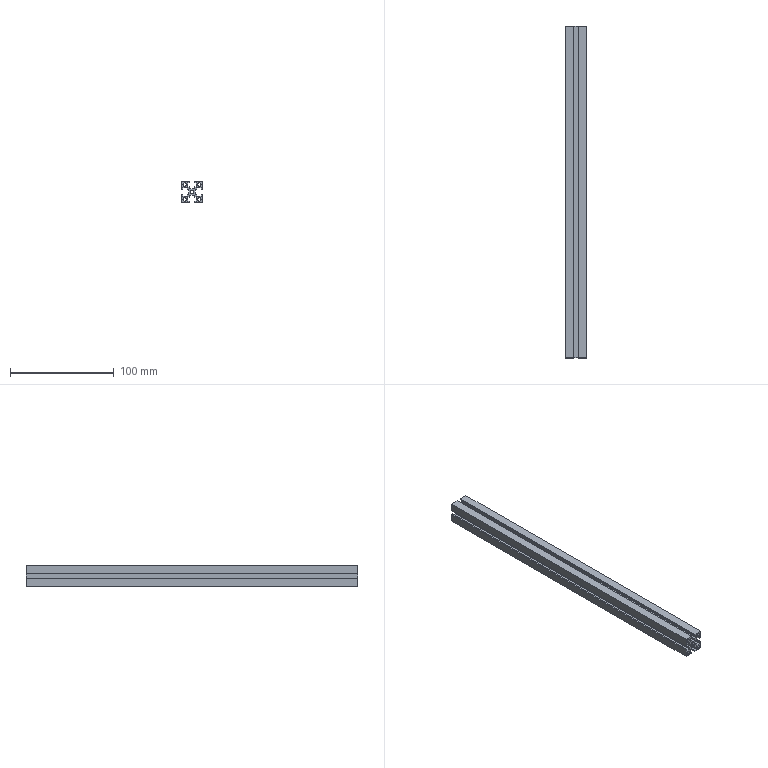Part | STEP file | 20 aluminium profile vertical 6 | 1 solid | 64 faces | box 20 x 320 x 20 mm | volume 56889 mm3 | plane 54 | cylinder 10 | commonest cylinder face diameters 3.3 x10